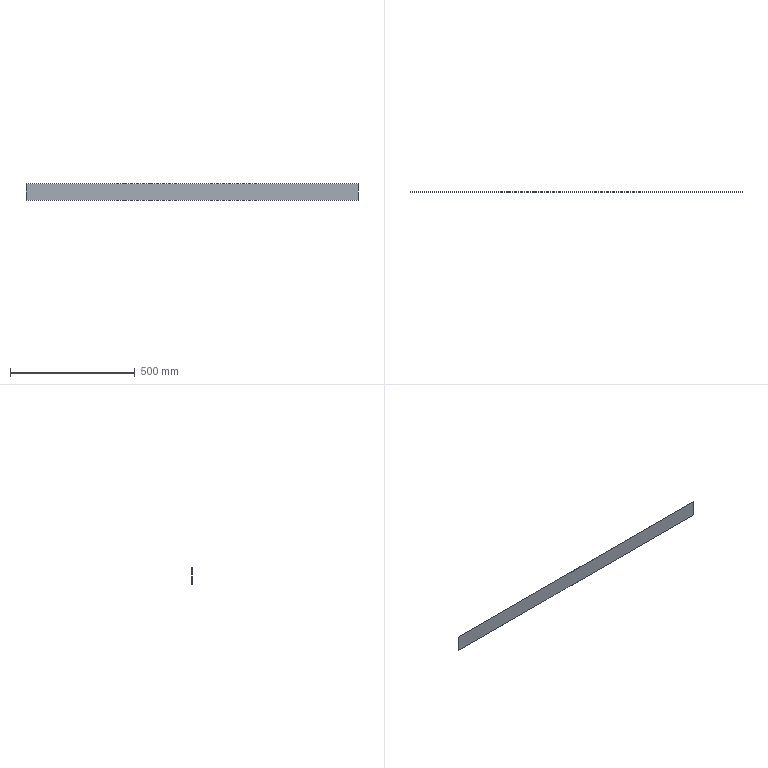Part | SolidWorks | features BaseBody 1 | 1 solid | 6 faces | box 1330 x 0.2 x 66 mm | volume 17556 mm3 | plane 6
STEP:
#1=CARTESIAN_POINT('',(-671.521,191.8,334.5));
#2=VERTEX_POINT('',#1);
#3=CARTESIAN_POINT('',(658.479,191.8,334.5));
#4=VERTEX_POINT('',#3);
#5=CARTESIAN_POINT('',(658.479,191.8,334.5));
#6=DIRECTION('',(1.,0.,0.));
#7=VECTOR('',#6,1000.);
#8=LINE('',#5,#7);
#9=EDGE_CURVE('',#2,#4,#8,.T.);
#10=ORIENTED_EDGE('',*,*,#9,.T.);
#11=CARTESIAN_POINT('',(658.479,191.8,400.5));
#12=VERTEX_POINT('',#11);
#13=CARTESIAN_POINT('',(658.479,191.8,400.5));
#14=DIRECTION('',(0.,0.,1.));
#15=VECTOR('',#14,1000.);
#16=LINE('',#13,#15);
#17=EDGE_CURVE('',#4,#12,#16,.T.);
#18=ORIENTED_EDGE('',*,*,#17,.T.);
#19=CARTESIAN_POINT('',(-671.521,191.8,400.5));
#20=VERTEX_POINT('',#19);
#21=CARTESIAN_POINT('',(658.479,191.8,400.5));
#22=DIRECTION('',(-1.,0.,0.));
#23=VECTOR('',#22,1000.);
#24=LINE('',#21,#23);
#25=EDGE_CURVE('',#12,#20,#24,.T.);
#26=ORIENTED_EDGE('',*,*,#25,.T.);
#27=CARTESIAN_POINT('',(-671.521,191.8,400.5));
#28=DIRECTION('',(0.,0.,-1.));
#29=VECTOR('',#28,1000.);
#30=LINE('',#27,#29);
#31=EDGE_CURVE('',#20,#2,#30,.T.);
#32=ORIENTED_EDGE('',*,*,#31,.T.);
#33=EDGE_LOOP('',(#10,#18,#26,#32));
#34=FACE_OUTER_BOUND('',#33,.T.);
#35=CARTESIAN_POINT('',(658.479,191.8,400.5));
#36=DIRECTION('',(0.,-1.,0.));
#37=DIRECTION('',(0.,0.,-1.));
#38=AXIS2_PLACEMENT_3D('',#35,#36,#37);
#39=PLANE('',#38);
#40=ADVANCED_FACE('',(#34),#39,.T.);
#41=CARTESIAN_POINT('',(658.479,192.,400.5));
#42=VERTEX_POINT('',#41);
#43=CARTESIAN_POINT('',(658.479,191.9,400.5));
#44=DIRECTION('',(0.,1.,0.));
#45=VECTOR('',#44,1000.);
#46=LINE('',#43,#45);
#47=EDGE_CURVE('',#12,#42,#46,.T.);
#48=ORIENTED_EDGE('',*,*,#47,.F.);
#49=ORIENTED_EDGE('',*,*,#17,.F.);
#50=CARTESIAN_POINT('',(658.479,192.,334.5));
#51=VERTEX_POINT('',#50);
#52=CARTESIAN_POINT('',(658.479,191.9,334.5));
#53=DIRECTION('',(0.,-1.,0.));
#54=VECTOR('',#53,1000.);
#55=LINE('',#52,#54);
#56=EDGE_CURVE('',#51,#4,#55,.T.);
#57=ORIENTED_EDGE('',*,*,#56,.F.);
#58=CARTESIAN_POINT('',(658.479,192.,367.5));
#59=DIRECTION('',(0.,0.,-1.));
#60=VECTOR('',#59,1000.);
#61=LINE('',#58,#60);
#62=EDGE_CURVE('',#42,#51,#61,.T.);
#63=ORIENTED_EDGE('',*,*,#62,.F.);
#64=EDGE_LOOP('',(#48,#49,#57,#63));
#65=FACE_OUTER_BOUND('',#64,.T.);
#66=CARTESIAN_POINT('',(658.479,191.9,367.5));
#67=DIRECTION('',(-1.,0.,0.));
#68=DIRECTION('',(0.,0.,1.));
#69=AXIS2_PLACEMENT_3D('',#66,#67,#68);
#70=PLANE('',#69);
#71=ADVANCED_FACE('',(#65),#70,.F.);
#72=CARTESIAN_POINT('',(-671.521,192.,334.5));
#73=VERTEX_POINT('',#72);
#74=CARTESIAN_POINT('',(658.479,192.,334.5));
#75=DIRECTION('',(1.,0.,0.));
#76=VECTOR('',#75,1000.);
#77=LINE('',#74,#76);
#78=EDGE_CURVE('',#73,#51,#77,.T.);
#79=ORIENTED_EDGE('',*,*,#78,.T.);
#80=ORIENTED_EDGE('',*,*,#56,.T.);
#81=ORIENTED_EDGE('',*,*,#9,.F.);
#82=CARTESIAN_POINT('',(-671.521,191.8,334.5));
#83=DIRECTION('',(0.,1.,0.));
#84=VECTOR('',#83,1000.);
#85=LINE('',#82,#84);
#86=EDGE_CURVE('',#2,#73,#85,.T.);
#87=ORIENTED_EDGE('',*,*,#86,.T.);
#88=EDGE_LOOP('',(#79,#80,#81,#87));
#89=FACE_OUTER_BOUND('',#88,.T.);
#90=CARTESIAN_POINT('',(658.479,191.8,334.5));
#91=DIRECTION('',(0.,0.,-1.));
#92=DIRECTION('',(-1.,0.,0.));
#93=AXIS2_PLACEMENT_3D('',#90,#91,#92);
#94=PLANE('',#93);
#95=ADVANCED_FACE('',(#89),#94,.T.);
#96=ORIENTED_EDGE('',*,*,#31,.F.);
#97=CARTESIAN_POINT('',(-671.521,192.,400.5));
#98=VERTEX_POINT('',#97);
#99=CARTESIAN_POINT('',(-671.521,191.9,400.5));
#100=DIRECTION('',(0.,1.,0.));
#101=VECTOR('',#100,1000.);
#102=LINE('',#99,#101);
#103=EDGE_CURVE('',#20,#98,#102,.T.);
#104=ORIENTED_EDGE('',*,*,#103,.T.);
#105=CARTESIAN_POINT('',(-671.521,192.,367.5));
#106=DIRECTION('',(0.,0.,-1.));
#107=VECTOR('',#106,1000.);
#108=LINE('',#105,#107);
#109=EDGE_CURVE('',#98,#73,#108,.T.);
#110=ORIENTED_EDGE('',*,*,#109,.T.);
#111=ORIENTED_EDGE('',*,*,#86,.F.);
#112=EDGE_LOOP('',(#96,#104,#110,#111));
#113=FACE_OUTER_BOUND('',#112,.T.);
#114=CARTESIAN_POINT('',(-671.521,191.9,367.5));
#115=DIRECTION('',(-1.,0.,0.));
#116=DIRECTION('',(0.,0.,1.));
#117=AXIS2_PLACEMENT_3D('',#114,#115,#116);
#118=PLANE('',#117);
#119=ADVANCED_FACE('',(#113),#118,.T.);
#120=ORIENTED_EDGE('',*,*,#25,.F.);
#121=ORIENTED_EDGE('',*,*,#47,.T.);
#122=CARTESIAN_POINT('',(658.479,192.,400.5));
#123=DIRECTION('',(-1.,0.,0.));
#124=VECTOR('',#123,1000.);
#125=LINE('',#122,#124);
#126=EDGE_CURVE('',#42,#98,#125,.T.);
#127=ORIENTED_EDGE('',*,*,#126,.T.);
#128=ORIENTED_EDGE('',*,*,#103,.F.);
#129=EDGE_LOOP('',(#120,#121,#127,#128));
#130=FACE_OUTER_BOUND('',#129,.T.);
#131=CARTESIAN_POINT('',(658.479,192.,400.5));
#132=DIRECTION('',(0.,0.,1.));
#133=DIRECTION('',(1.,0.,0.));
#134=AXIS2_PLACEMENT_3D('',#131,#132,#133);
#135=PLANE('',#134);
#136=ADVANCED_FACE('',(#130),#135,.T.);
#137=ORIENTED_EDGE('',*,*,#126,.F.);
#138=ORIENTED_EDGE('',*,*,#62,.T.);
#139=ORIENTED_EDGE('',*,*,#78,.F.);
#140=ORIENTED_EDGE('',*,*,#109,.F.);
#141=EDGE_LOOP('',(#137,#138,#139,#140));
#142=FACE_OUTER_BOUND('',#141,.T.);
#143=CARTESIAN_POINT('',(658.479,192.,334.5));
#144=DIRECTION('',(0.,1.,0.));
#145=DIRECTION('',(0.,0.,1.));
#146=AXIS2_PLACEMENT_3D('',#143,#144,#145);
#147=PLANE('',#146);
#148=ADVANCED_FACE('',(#142),#147,.T.);
#149=CLOSED_SHELL('',(#40,#71,#95,#119,#136,#148));
#150=MANIFOLD_SOLID_BREP('',#149);
#151=CARTESIAN_POINT('',(0.,0.,0.));
#152=DIRECTION('',(0.,0.,1.));
#153=DIRECTION('',(1.,0.,0.));
#154=AXIS2_PLACEMENT_3D('',#151,#152,#153);
#155=(LENGTH_UNIT()NAMED_UNIT(*)SI_UNIT(.MILLI.,.METRE.));
#156=UNCERTAINTY_MEASURE_WITH_UNIT(LENGTH_MEASURE(0.00001),#155,'','');
#157=(NAMED_UNIT(*)PLANE_ANGLE_UNIT()SI_UNIT($,.RADIAN.));
#158=(NAMED_UNIT(*)SI_UNIT($,.STERADIAN.)SOLID_ANGLE_UNIT());
#159=(GEOMETRIC_REPRESENTATION_CONTEXT(3)GLOBAL_UNCERTAINTY_ASSIGNED_CONTEXT((#156))GLOBAL_UNIT_ASSIGNED_CONTEXT((#155,#157,#158))REPRESENTATION_CONTEXT('',''));
#160=ADVANCED_BREP_SHAPE_REPRESENTATION('',(#150,#154),#159);